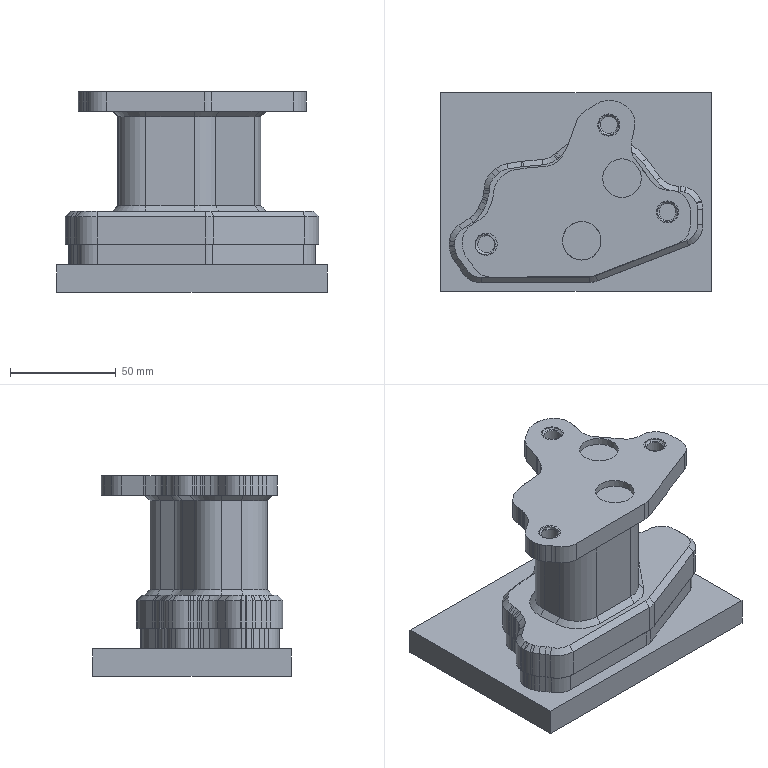NC program | NX | posted by the shop | part box 128.162 x 94.109 x 95 mm
Lines 1 to 893 of 2518:
1 BEGIN PGM B MM
2 BLK FORM 0.1 Z X-200 Y-200 Z-20
3 BLK FORM 0.2  X+200  Y+200  Z+0
4 CYCL DEF 247 DATUM SETTING ~
Q339=+1
5 * - OPERATION: 动态开粗_1_COPY - TOOL: T18 C-D10
6 M5
7 M9
8 PLANE RESET STAY
9 CALL LBL100
10 ;(C-D10 D=10. R=0.)
11 M01
12 TOOL CALL 18 Z S7000
13 CALL LBL101
14 M3 M8
15 M51
16 CYCL DEF 7.0
17 CYCL DEF 7.1 X0
18 CYCL DEF 7.2 Y0
19 CYCL DEF 7.3 Z0
20 CYCL DEF 32.0 TOLERANCE
21 CYCL DEF 32.1 T0.096
22 CYCL DEF 32.2 HSC-MODE:0
23 L M126
24 L A+0.0 C+0.0 FMAX
25 L X65.5231 Y54.6487 FMAX
26 L Z100.1 FMAX
27 L Z85.1 FMAX
28 L Z82.1 F4000.
29 L X65.3697 Y53.0086
30 CC X66.3796 Y52.9169
31 C X65.908 Y52.0191 DR+
32 CC X59.8991 Y27.7131
33 C X68.5518 Y51.2082 DR-
34 CC X64.826 Y44.4706
35 C X72.2902 Y46.3579 DR-
36 CC X43.8286 Y39.0382
37 C X73.2137 Y38.6371 DR-
38 L X73.2796 Y29.0376
39 L X73.2534 Y-44.7659
40 CC X67.0232 Y-43.8302
41 C X69.4184 Y-49.6572 DR-
42 CC X70.3761 Y-52.7478
43 C X67.7081 Y-50.9173 DR+
44 CC X63.6112 Y-46.2833
45 C X65.842 Y-52.0524 DR-
46 CC X66.2949 Y-52.944
47 C X66.2119 Y-53.9406 DR+
48 L X66.8127 Y-53.8771 Z82.2533
49 L X67.4061 Y-53.7642 Z82.4066
50 L X68.1568 Y-53.6324 Z82.6
51 L X69.8793 Y-53.3203 F15000.
52 L X70.1271 Y-53.2006
53 L X72.8269 Y-51.3837
54 CC X68.1598 Y-45.2629
55 C X75.2625 Y-48.229 DR+
56 CC X64.7277 Y-43.3664
57 C X76.3295 Y-43.5273 DR+
58 L X77.2543 Y25.4765
59 CC X-25.2401 Y26.8347
60 C X76.3881 Y40.2005 DR+
61 L X75.6476 Y45.7172
62 CC X62.7408 Y43.3635
63 C X73.232 Y51.2414 DR+
64 CC X65.6303 Y45.2338
65 C X71.4123 Y53.0085 DR+
66 L X69.6105 Y54.3237
67 CC X69.1482 Y53.3821
68 C X68.9718 Y54.4161 DR+
69 L X67.3131 Y54.1061
70 L X66.0198 Y53.8508 Z82.2652 F4000.
71 CC X66.4053 Y52.8551
72 CP IPA34.9502 IZ-.1652 DR+
73 CC X66.3619 Y52.911
74 C X65.908 Y52.0191 DR+
75 CC X62.1689 Y43.8151
76 C X70.2548 Y47.8032 DR-
77 CC X52.9069 Y39.3043
78 C X72.2083 Y40.1037 DR-
79 CC X-136.0307 Y29.0316
80 C X72.4791 Y25.9096 DR-
81 L X72.4538 Y-42.3025
82 CC X64.2353 Y-41.3322
83 C X69.9435 Y-47.3239 DR-
84 CC X71.2981 Y-49.0395
85 C X69.1919 Y-48.4547 DR+
86 CC X62.6392 Y-46.3457
87 C X68.3045 Y-50.256 DR-
88 CC X69.14 Y-50.8056
89 C X69.4411 Y-51.7593 DR+
90 L X69.827 Y-51.5366 Z82.2132
91 L X70.1633 Y-51.2443 Z82.3263
92 L X70.98 Y-50.5415 Z82.6
93 L X72.5067 Y-49.2155 F15000.
94 L X74.4022 Y-46.3635
95 CC X68.1042 Y-42.7162
96 C X75.3794 Y-42.914 DR+
97 L X75.9502 Y-20.9168
98 CC X-709.6475 Y-4.5601
99 C X75.8982 Y14.1254 DR+
100 L X75.1833 Y44.0744
101 CC X67.9863 Y43.899
102 C X73.9781 Y47.8898 DR+
103 L X71.6313 Y51.3912
104 L X71.4675 Y51.528
105 L X71.2861 Y51.6404
106 L X69.7372 Y52.315
107 L X68.2309 Y52.9559 Z82.1844 F4000.
108 L X67.8994 Y52.9814 Z82.1
109 CC X67.9898 Y51.9853
110 C X67.2824 Y51.2783 DR+
111 CC X62.923 Y46.1428
112 C X69.3811 Y48.0589 DR-
113 CC X39.2885 Y36.5453
114 C X71.5034 Y37.12 DR-
115 CC X-338.6129 Y24.7933
116 C X71.6792 Y22.0224 DR-
117 L X71.6451 Y-40.2768
118 CC X58.7607 Y-38.7741
119 C X69.6144 Y-45.8779 DR-
120 CC X71.4265 Y-46.8913
121 C X69.377 Y-47.2235 DR+
122 L X69.1986 Y-48.4101
123 CC X70.1878 Y-48.5585
124 C X70.498 Y-49.5094 DR+
125 CC X70.0128 Y-48.3113
126 CP IPA42.1022 IZ.2409 DR+
127 L X71.7352 Y-48.0227 Z82.6
128 L X72.4667 Y-46.8889 F15000.
129 L X72.5288 Y-46.6825
130 L X72.5603 Y-46.4692
131 L X72.8284 Y47.8111
132 CC X71.8193 Y47.8092
133 C X72.3949 Y48.638 DR+
134 L X71.5444 Y49.2227
135 L X70.4736 Y49.9413 Z82.2724 F4000.
136 CC X70.0492 Y48.9699
137 CP IPA36.7473 IZ-.1724 DR+
138 CC X70.0563 Y49.0323
139 C X69.0789 Y48.8158 DR+
140 CC X-21.6563 Y30.7456
141 C X70.8549 Y29.7066 DR-
142 L X70.8456 Y-38.3927
143 CC X51.6289 Y-36.657
144 C X69.3892 Y-44.198 DR-
145 L X69.3771 Y-46.5972
146 CC X70.3778 Y-46.5964
147 C X70.4616 Y-47.5937 DR+
148 CC X70.3344 Y-46.5054
149 CP IPA55.2046 IZ.2676 DR+
150 L X71.826 Y-46.2733 Z82.6
151 L X72.6354 Y-45.0995 F15000.
152 L X72.7059 Y-44.8823
153 L X72.7388 Y-44.6563
154 L X72.7032 Y45.7946
155 L X72.6372 Y46.011
156 L X72.5363 Y46.2135
157 L X71.8357 Y47.223
158 L X71.0714 Y48.3014 Z82.2643 F4000.
159 CC X70.3195 Y47.5417
160 CP IPA34.7263 IZ-.1643 DR+
161 CC X70.3534 Y47.6053
162 C X69.353 Y47.5845 DR+
163 CC X194.1957 Y48.0079
164 C X69.8207 Y37.2036 DR+
165 CC X-355.6725 Y21.8096
166 C X70.0783 Y17.6074 DR-
167 L X70.0509 Y-36.5922
168 CC X46.6757 Y-35.3927
169 C X69.3772 Y-41.0917 DR-
170 L X69.3771 Y-44.3917
171 CC X70.3771 Y-44.3916
172 C X71.3142 Y-44.7408 DR+
173 L X71.8334 Y-42.8388 Z82.6
174 L X72.0023 Y-42.2488 F15000.
175 L X72.122 Y-41.6468
176 L X72.7411 Y42.1123
177 L X72.6928 Y42.4173
178 L X72.5587 Y42.6955
179 L X71.8363 Y43.7213
180 L X71.0861 Y44.7607 Z82.2744 F4000.
181 CC X70.3531 Y43.9974
182 CP IPA37.2271 IZ-.1744 DR+
183 CC X70.3802 Y44.0524
184 C X69.3794 Y44.0532 DR+
185 L X69.3772 Y-41.1468
186 CC X70.3876 Y-41.1462
187 C X70.6862 Y-42.1115 DR+
188 L X71.1865 Y-41.9481
189 L X71.699 Y-41.828
190 CC X71.7599 Y-42.8361
191 C X71.8408 Y-43.8429 DR-
192 L Z85.1
193 L Z100.1 FMAX
194 L X-63.991 Y-54.784 FMAX
195 L Z85.1 FMAX
196 L Z82.1
197 CC X-64.1911 Y-53.793
198 C X-65.1854 Y-53.9757 DR-
199 L X-65.3121 Y-53.2387
200 L X-65.4789 Y-52.5097
201 CC X-66.4514 Y-52.9474
202 C X-65.9277 Y-52.0184 DR+
203 CC X-57.4511 Y-19.1989
204 C X-68.444 Y-51.2633 DR-
205 CC X-64.7635 Y-44.4368
206 C X-72.2791 Y-46.3506 DR-
207 CC X-43.4503 Y-38.9275
208 C X-73.2153 Y-38.4311 DR-
209 L X-73.2769 Y-29.2315
210 L X-73.2395 Y44.8736
211 CC X-67.0453 Y43.8397
212 C X-69.4858 Y49.626 DR-
213 L X-68.3627 Y50.1762
214 CC X-63.5742 Y46.3859
215 C X-65.9042 Y52.031 DR-
216 CC X-66.3695 Y52.9163
217 C X-66.1448 Y53.8908 DR+
218 L X-66.5885 Y53.8959 Z82.2127
219 L X-67.0252 Y53.8171 Z82.3254
220 L X-68.0904 Y53.6314 Z82.6
221 L X-69.9407 Y53.2992 F15000.
222 L X-70.1894 Y53.1793
223 L X-72.8892 Y51.3624
224 CC X-68.2221 Y45.2416
225 C X-75.3248 Y48.2077 DR+
226 CC X-64.79 Y43.345
227 C X-76.3918 Y43.506 DR+
228 L X-77.267 Y-21.8012
229 CC X59.057 Y-23.611
230 C X-76.408 Y-38.9977 DR+
231 L X-75.6237 Y-45.7678
232 CC X-63.6667 Y-43.8711
233 C X-72.9547 Y-51.6365 DR+
234 CC X-65.6826 Y-45.1881
235 C X-71.4485 Y-53.0123 DR+
236 L X-69.6306 Y-54.3216
237 CC X-69.1731 Y-53.3761
238 C X-68.9954 Y-54.4113 DR+
239 L X-67.3484 Y-54.1012
240 L X-66.0515 Y-53.8436 Z82.2641 F4000.
241 CC X-66.438 Y-52.8469
242 CP IPA34.6972 IZ-.1641 DR+
243 CC X-66.3939 Y-52.9039
244 C X-65.9277 Y-52.0184 DR+
245 CC X-62.0364 Y-43.7205
246 C X-70.2418 Y-47.8031 DR-
247 CC X-52.5413 Y-39.1616
248 C X-72.228 Y-39.8081 DR-
249 CC X191.8602 Y-27.6687
250 C X-72.4772 Y-23.7132 DR-
251 L X-72.4512 Y42.3108
252 CC X-64.3707 Y41.3836
253 C X-70.0232 Y47.2319 DR-
254 CC X-71.5034 Y49.1883
255 C X-69.0786 Y48.8158 DR+
256 CC X-42.6537 Y35.2732
257 C X-68.2967 Y50.2435 DR-
258 CC X-69.0109 Y50.9435
259 C X-69.4178 Y51.857 DR+
260 L X-69.8212 Y51.5726 Z82.2253
261 L X-70.1874 Y51.2416 Z82.3506
262 L X-70.9262 Y50.5935 Z82.6
263 L X-72.5021 Y49.1995 F15000.
264 L X-74.3944 Y46.3512
265 CC X-68.0946 Y42.7028
266 C X-75.3718 Y42.9013 DR+
267 L X-75.943 Y21.413
268 CC X654.4759 Y2.0349
269 C X-75.8641 Y-20.1183 DR+
270 L X-75.105 Y-45.1039
271 CC X-68.9945 Y-44.9149
272 C X-73.897 Y-48.5672 DR+
273 L X-72.9778 Y-49.8177
274 L X-72.0295 Y-51.0462
275 L X-71.7428 Y-51.2359
276 L X-70.1183 Y-51.9453
277 L X-68.7169 Y-52.5452 Z82.2129 F4000.
278 L X-68.4962 Y-52.571 Z82.1564
279 L X-68.2742 Y-52.5627 Z82.1
280 CC X-68.4575 Y-51.5794
281 C X-67.7078 Y-50.9173 DR+
282 CC X-62.6154 Y-46.0911
283 C X-69.3424 Y-48.0843 DR-
284 CC X-39.7381 Y-36.5681
285 C X-71.4981 Y-37.1511 DR-
286 CC X335.7578 Y-24.7604
287 C X-71.6769 Y-21.9536 DR-
288 L X-71.6452 Y40.2458
289 CC X-59.5197 Y38.9909
290 C X-69.7285 Y45.653 DR-
291 CC X-72.3691 Y47.169
292 C X-69.3527 Y47.5845 DR+
293 L X-69.1789 Y48.3654
294 CC X-70.1552 Y48.5825
295 C X-70.5905 Y49.4829 DR+
296 CC X-69.8911 Y48.2692
297 CP IPA34.0662 IZ.2112 DR+
298 L X-71.7638 Y47.9255 Z82.6
299 L X-72.4502 Y46.8357 F15000.
300 L X-72.5094 Y46.6332
301 L X-72.5406 Y46.4245
302 L X-72.9412 Y-47.4501
303 CC X-71.933 Y-47.4499
304 C X-72.4877 Y-48.2917 DR+
305 L X-71.6634 Y-48.8298
306 L X-70.5768 Y-49.5216 Z82.2728 F4000.
307 CC X-70.1763 Y-48.5404
308 CP IPA36.8374 IZ-.1728 DR+
309 CC X-70.1822 Y-48.6023
310 C X-69.1916 Y-48.4547 DR+
311 CC X122.4897 Y-16.6918
312 C X-70.4983 Y-39.192 DR-
313 CC X119.3213 Y-27.0395
314 C X-70.8737 Y-24.8009 DR-
315 L X-70.8433 Y38.3985
316 CC X-50.738 Y36.4406
317 C X-69.3862 Y44.2058 DR-
318 L X-69.3749 Y46.5532
319 CC X-70.3757 Y46.5627
320 C X-70.4256 Y47.5623 DR+
321 CC X-70.3329 Y46.4685
322 CP IPA57.5196 IZ.2794 DR+
323 L X-71.8021 Y46.2658 Z82.6
324 L X-72.634 Y45.0535 F15000.
325 L X-72.7039 Y44.8372
326 L X-72.7366 Y44.6123
327 L X-72.7269 Y-45.4349
328 L X-72.6599 Y-45.6531
329 L X-72.5571 Y-45.8569
330 L X-71.8597 Y-46.8509
331 L X-71.0913 Y-47.9231 Z82.265 F4000.
332 CC X-70.3444 Y-47.1598
333 CP IPA34.9007 IZ-.165 DR+
334 CC X-70.3774 Y-47.2227
335 C X-69.3768 Y-47.2235 DR+
336 CC X-162.5223 Y-46.5544
337 C X-69.7778 Y-37.8945 DR+
338 CC X322.9775 Y-21.9083
339 C X-70.076 Y-17.2995 DR-
340 L X-70.0483 Y36.6002
341 CC X-46.8827 Y35.4081
342 C X-69.3791 Y41.0631 DR-
343 L Y44.3631
344 CC X-70.3792 Y44.3629
345 C X-71.2802 Y44.7968 DR+
346 L X-71.5585 Y43.8514 Z82.35
347 L X-71.8114 Y42.8989 Z82.6
348 L X-72.1148 Y41.7463 F15000.
349 L X-72.7386 Y-42.0826
350 L X-72.6902 Y-42.3875
351 L X-72.5562 Y-42.6657
352 L X-71.8582 Y-43.6568
353 L X-71.0896 Y-44.7249 Z82.2658 F4000.
354 CC X-70.3452 Y-43.9605
355 CP IPA35.1027 IZ-.1658 DR+
356 CC X-70.3775 Y-44.0227
357 C X-69.3769 Y-44.0235 DR+
358 L X-69.3791 Y41.0765
359 CC X-70.3906 Y41.0751
360 C X-70.2437 Y42.076 DR+
361 L X-71.8187 Y42.305
362 L Z85.1
363 L Z100.1 FMAX
364 PLANE RESET STAY
365 * - OPERATION: 动态开粗_1 - TOOL: T18 C-D10
366 CYCL DEF 32.0 TOLERANCE
367 CYCL DEF 32.1 T0.096
368 CYCL DEF 32.2 HSC-MODE:0
369 L A+0.0 C+0.0 FMAX
370 L X71.6405 Y1.4365 FMAX
371 L Z100. FMAX
372 L Z75.5361 FMAX
373 L Z72.5361 F4000.
374 L X69.6182 Y.4541
375 CC X70.1084 Y-.5042
376 C X69.1596 Y.0041 DR+
377 CC X79.1767 Y-3.8411
378 C X68.447 Y-3.8787 DR+
379 CC X361.5552 Y-13.7916
380 C X68.2801 Y-14.4035 DR+
381 L X68.2535 Y-44.7659
382 CC X62.0101 Y-43.8266
383 C X64.4238 Y-49.6607 DR-
384 CC X57.2669 Y-32.5753
385 C X57.4167 Y-51.0985 DR-
386 CC X47.0047 Y296.47
387 C X45.619 Y-51.2516 DR-
388 L X-61.9391 Y-51.212
389 CC X-60.7765 Y-44.9278
390 C X-66.6716 Y-47.3956 DR-
391 CC X-49.8833 Y-40.2742
392 C X-68.1183 Y-40.4897 DR-
393 CC X282.7887 Y-29.4374
394 C X-68.28 Y-26.4921 DR-
395 L X-68.2418 Y44.8737
396 CC X-61.9527 Y43.7878
397 C X-64.3299 Y49.7107 DR-
398 CC X-57.2383 Y32.335
399 C X-57.4121 Y51.1014 DR-
400 CC X-46.9584 Y-302.6918
401 C X-45.6143 Y51.2532 DR-
402 L X61.8004 Y51.227
403 CC X60.8663 Y45.0048
404 C X66.6494 Y47.4835 DR-
405 CC X49.8278 Y40.2787
406 C X68.1271 Y40.3857 DR-
407 CC X-282.7002 Y29.9586
408 C X68.2793 Y28.5879 DR-
409 L X68.249 Y2.3886
410 CC X198.4264 Y-11.8206
411 C X67.4868 Y-13.5142 DR+
412 L X67.4539 Y-42.3026
413 CC X59.6658 Y-41.4074
414 C X62.6904 Y-48.6398 DR-
415 CC X54.5689 Y-29.2309
416 C X54.9086 Y-50.2677 DR-
417 CC X44.3375 Y244.9354
418 C X42.5115 Y-50.4513 DR-
419 L X-59.3761 Y-50.4204
420 CC X-58.3699 Y-42.5497
421 C X-65.7345 Y-45.503 DR-
422 CC X-45.4319 Y-37.3485
423 C X-67.3095 Y-37.6029 DR-
424 CC X261.3603 Y-26.9474
425 C X-67.479 Y-25.5054 DR-
426 L X-67.4533 Y42.3108
427 CC X-59.6835 Y41.4196
428 C X-62.7468 Y48.6155 DR-
429 CC X-54.7168 Y29.807
430 C X-55.1704 Y50.2529 DR-
431 CC X-43.5644 Y-256.7811
432 C X-40.1739 Y50.4535 DR-
433 L X59.3369 Y50.4268
434 CC X58.4393 Y42.6413
435 C X65.6704 Y45.6631 DR-
436 CC X46.2537 Y37.5472
437 C X67.2957 Y37.8801 DR-
438 CC X-247.5041 Y26.8258
439 C X67.4794 Y24.283 DR-
440 CC X-847.4335 Y16.3748
441 C X67.4202 Y3.2976 DR-
442 CC X300.432 Y-15.6072
443 C X66.6792 Y-19.0031 DR+
444 CC X-911.3933 Y-27.7345
445 C X66.6361 Y-40.402 DR-
446 CC X57.7611 Y-39.502
447 C X61.067 Y-47.7874 DR-
448 CC X52.2992 Y-25.7183
449 C X52.6809 Y-49.4622 DR-
450 CC X41.5999 Y263.7296
451 C X39.4838 Y-49.651 DR-
452 L X-57.2156 Y-49.6228
453 CC X-56.5163 Y-40.7134
454 C X-64.8381 Y-43.9714 DR-
455 CC X-42.3082 Y-35.158
456 C X-66.4985 Y-35.4797 DR-
457 CC X285.409 Y-23.9192
458 C X-66.6792 Y-21.3824 DR-
459 L X-66.643 Y40.3167
460 CC X-57.7969 Y39.5269
461 C X-61.1651 Y47.7448 DR-
462 CC X-52.3747 Y26.0973
463 C X-52.783 Y49.4579 DR-
464 CC X-40.6821 Y-295.902
465 C X-37.2861 Y49.6531 DR-
466 L X57.3131 Y49.619
467 CC X56.5339 Y40.7317
468 C X64.8382 Y43.9921 DR-
469 CC X42.3393 Y35.1845
470 C X66.4986 Y35.5013 DR-
471 CC X-287.0018 Y23.9034
472 C X66.6792 Y21.304 DR-
473 CC X-469.0986 Y15.3826
474 C X66.5779 Y3.3985 DR-
475 CC X345.3128 Y-16.5419
476 C X65.8802 Y-19.4051 DR+
477 CC X-793.8738 Y-26.5384
478 C X65.8238 Y-38.7028 DR-
479 CC X56.1711 Y-37.8919
480 C X59.7658 Y-46.8869 DR-
481 CC X50.5117 Y-23.4883
482 C X50.9853 Y-48.646 DR-
483 CC X38.7119 Y291.3707
484 C X35.3886 Y-48.8512 DR-
485 L X-55.4108 Y-48.8167
486 CC X-54.9003 Y-39.1249
487 C X-63.9103 Y-42.7324 DR-
488 CC X-40.5069 Y-33.469
489 C X-65.6722 Y-33.9543 DR-
490 CC X269.3953 Y-21.7378
491 C X-65.8788 Y-18.4576 DR-
492 L X-65.8425 Y38.4417
493 CC X-56.1393 Y37.878
494 C X-59.6337 Y46.9477 DR-
495 CC X-50.527 Y23.3661
496 C X-51.1379 Y48.6377 DR-
497 CC X-38.8269 Y-276.9229
498 C X-35.4415 Y48.8527 DR-
499 L X55.358 Y48.8227
500 CC X54.9163 Y39.142
501 C X63.9203 Y42.7252 DR-
502 CC X40.2638 Y33.4225
503 C X65.6801 Y33.848 DR-
504 CC X-244.6344 Y22.5882
505 C X65.8783 Y20.6511 DR-
506 CC X-310.8721 Y15.2421
507 C X65.7034 Y2.5543 DR-
508 CC X376.7183 Y-17.2407
509 C X65.0803 Y-19.2049 DR+
510 CC X-541.9694 Y-25.8315
511 C X65.01 Y-37.2021 DR-
512 CC X54.6518 Y-36.3917
513 C X58.2574 Y-46.1358 DR-
514 CC X48.6537 Y-20.1548
515 C X49.1623 Y-47.8493 DR-
516 CC X36.6826 Y312.8662
517 C X33.4654 Y-48.0508 DR-
518 L X-53.7764 Y-48.0118
519 CC X-53.4082 Y-37.6336
520 C X-63.1024 Y-41.3574 DR-
521 CC X-37.8116 Y-31.7301
522 C X-64.8673 Y-32.2743 DR-
523 CC X285.8471 Y-19.6023
524 C X-65.0785 Y-16.0776 DR-
525 L X-65.0522 Y36.522
526 CC X-54.6596 Y36.3818
527 C X-58.3547 Y46.0964 DR-
528 CC X-48.9233 Y21.3095
529 C X-49.6669 Y47.8196 DR-
530 CC X-37.0838 Y-265.7701
531 C X-33.5709 Y48.0523 DR-
532 L X53.7285 Y48.0172
533 CC X53.3948 Y37.5984
534 C X63.1948 Y41.1511 DR-
535 CC X37.1927 Y31.648
536 C X64.8705 Y32.2429 DR-
537 CC X-406.1117 Y17.0858
538 C X64.9023 Y2.949 DR-
539 CC X434.7168 Y-18.6577
540 C X64.2797 Y-21.104 DR+
541 CC X-327.6751 Y-26.278
542 C X64.1981 Y-35.802 DR-
543 CC X53.2956 Y-35.0272
544 C X57.0494 Y-45.2924 DR-
545 CC X47.2454 Y-18.5641
546 C X47.9538 Y-47.025 DR-
547 CC X34.9944 Y294.2995
548 C X31.2575 Y-47.2505 DR-
549 L X-52.142 Y-47.2134
550 CC X-52.0155 Y-36.245
551 C X-62.3027 Y-40.0524 DR-
552 CC X-35.9286 Y-30.2827
553 C X-64.0433 Y-31.0612 DR-
554 CC X262.9895 Y-18.088
555 C X-64.2781 Y-14.2652 DR-
556 L X-64.2459 Y35.0344
557 CC X-53.2276 Y34.9686
558 C X-56.8531 Y45.3737 DR-
559 CC X-47.063 Y17.5699
560 C X-47.7406 Y47.0391 DR-
561 CC X-34.8243 Y-314.5893
562 C X-31.2439 Y47.252 DR-
563 L X52.0557 Y47.2198
564 CC X52.0018 Y36.2185
565 C X62.3639 Y39.9143 DR-
566 CC X34.6968 Y30.0291
567 C X64.071 Y30.6122 DR-
568 CC X-356.0922 Y16.689
569 C X63.676 Y-6.2379 DR-
570 CC X1030.0374 Y-27.5321
571 C X63.4581 Y-33.2027 DR+
572 CC X51.7056 Y-33.5522
573 C X60.2182 Y-41.6626 DR-
574 CC X49.7455 Y-30.2677
575 C X52.1134 Y-45.5619 DR-
576 CC X41.442 Y20.6017
577 C X40.5599 Y-46.4112 DR-
578 L X-50.5395 Y-46.417
579 CC X-50.6823 Y-34.9175
580 C X-61.5127 Y-38.7855 DR-
581 CC X-32.9212 Y-28.6173
582 C X-63.2596 Y-29.2833 DR-
583 CC X291.5364 Y-16.4281
584 C X-63.4777 Y-13.1867 DR-
585 L X-63.4414 Y33.6128
586 CC X-51.9458 Y33.6678
587 C X-55.7452 Y44.5175 DR-
588 CC X-45.543 Y15.3381
589 C X-46.1387 Y46.2439 DR-
590 CC X-33.3256 Y-326.0479
591 C X-30.2418 Y46.4515 DR-
592 L X50.4579 Y46.4227
593 CC X50.6885 Y34.9388
594 C X61.4621 Y38.9215 DR-
595 CC X33.9225 Y28.8366
596 C X63.2398 Y29.6298 DR-
597 CC X-313.6544 Y15.6733
598 C X62.9174 Y-5.2478 DR-
599 CC X935.9996 Y-27.1249
600 C X62.6559 Y-31.804 DR+
601 CC X49.9196 Y-32.1673
602 C X60.0929 Y-39.8387 DR-
603 CC X49.27 Y-30.3996
604 C X52.182 Y-44.462 DR-
605 CC X41.6325 Y5.394
606 C X41.4591 Y-45.5656 DR-
607 L X30.0597 Y-45.6491
608 L X-49.04 Y-45.619
609 CC X-49.2963 Y-33.2532
610 C X-57.3458 Y-42.6439 DR-
611 CC X-46.8069 Y-31.8913
612 C X-61.6132 Y-34.6223 DR-
613 CC X-4.3421 Y-23.8321
614 C X-62.6183 Y-23.2859 DR-
615 L X-62.6768 Y-12.9863
616 L X-62.6396 Y32.2133
617 CC X-50.6598 Y32.3998
618 C X-58.8849 Y41.1118 DR-
619 CC X-48.1931 Y28.2889
620 C X-50.4794 Y44.8272 DR-
621 CC X-39.1036 Y-34.4531
622 C X-37.7184 Y45.6272 DR-
623 L X49.281 Y45.6115
624 CC X49.4431 Y33.6815
625 C X58.3389 Y41.6323 DR-
626 CC X44.9508 Y31.0166
627 C X61.8901 Y33.251 DR-
628 CC X-21.2412 Y21.848
629 C X62.6559 Y20.3874 DR-
630 CC X-377.633 Y16.4874
631 C X62.0968 Y-6.0333 DR-
632 CC X981.3229 Y-27.6815
633 C X61.8469 Y-30.704 DR+
634 CC X48.6497 Y-30.9713
635 C X59.308 Y-38.7584 DR-
636 CC X48.1221 Y-29.2703
637 C X51.0547 Y-43.6421 DR-
638 CC X40.1832 Y8.2559
639 C X39.9333 Y-44.7679 DR-
640 L X26.6339 Y-44.8493
641 L X-47.6658 Y-44.8184
642 CC X-47.9644 Y-31.5243
643 C X-55.672 Y-42.3602 DR-
644 CC X-46.5225 Y-31.2376
645 C X-60.5862 Y-34.3417 DR-
646 CC X-12.1363 Y-23.4971
647 C X-61.7848 Y-23.3298 DR-
648 L X-61.8764 Y-11.6305
649 L X-61.8491 Y30.5693
650 CC X-48.4572 Y30.9147
651 C X-59.4481 Y38.5739 DR-
652 CC X-48.315 Y29.5728
653 C X-51.4199 Y43.5486 DR-
654 CC X-40.6281 Y-4.1281
655 C X-40.51 Y44.7546 DR-
656 CC X-29.0089 Y-609.9626
657 C X-26.5107 Y44.8508 DR-
658 L X47.6889 Y44.8197
659 CC X47.9911 Y31.6199
660 C X55.8412 Y42.236 DR-
661 CC X46.3647 Y31.1485
662 C X60.6318 Y34.1794 DR-
663 CC X9.5629 Y23.2039
664 C X61.7968 Y22.8628 DR-
665 CC X-389.3944 Y16.017
666 C X61.2903 Y-6.4262 DR-
667 CC X939.4913 Y-27.2504
668 C X61.046 Y-29.4042 DR+
669 CC X47.028 Y-29.6976
670 C X58.7174 Y-37.4402 DR-
671 CC X47.2692 Y-28.5722
672 C X50.425 Y-42.7053 DR-
673 CC X39.4073 Y5.501
674 C X39.3184 Y-43.9482 DR-
675 CC X28.0931 Y580.0297
676 C X27.0191 Y-44.0483 DR-
677 L X-46.3806 Y-44.0168
678 CC X-46.6798 Y-29.8021
679 C X-54.1827 Y-41.879 DR-
680 CC X-45.9093 Y-30.4482
681 C X-59.6046 Y-33.8473 DR-
682 CC X-16.4387 Y-23.0031
683 C X-60.9451 Y-23.2586 DR-
684 CC X558.8359 Y-10.5257
685 C X-61.0759 Y-10.3598 DR-
686 L X-61.0387 Y29.5398
687 CC X-47.3587 Y29.7895
688 C X-58.5096 Y37.718 DR-
689 CC X-47.0938 Y28.2933
690 C X-50.1577 Y42.7763 DR-
691 CC X-38.9683 Y-9.149
692 C X-38.6432 Y43.9673 DR-
693 L X-27.4438 Y44.0497
694 L X46.5558 Y44.0127
695 CC X46.8055 Y30.2911
696 C X54.7334 Y41.4934 DR-
697 CC X45.4529 Y30.1674
698 C X59.7439 Y33.3572 DR-
699 CC X9.823 Y22.1391
700 C X60.988 Y21.8502 DR-
701 CC X-362.3882 Y15.2924
702 C X60.5166 Y-5.7305 DR-
703 CC X1010.6387 Y-28.8292
704 C X60.2359 Y-28.4048 DR+
705 CC X46.0104 Y-28.6173
706 C X57.782 Y-36.6072 DR-
707 CC X46.2282 Y-27.5175
708 C X49.5626 Y-41.8351 DR-
709 CC X38.6049 Y4.1505
710 C X38.8642 Y-43.1219 DR-
711 CC X26.3533 Y577.9921
712 C X25.9654 Y-43.2478 DR-
713 L X-45.0344 Y-43.2181
714 CC X-45.4098 Y-28.0985
715 C X-52.9737 Y-41.1955 DR-
716 CC X-45.0481 Y-29.5211
717 C X-58.7079 Y-33.059 DR-
718 CC X-16.7459 Y-22.037
719 C X-60.1299 Y-22.3801 DR-
720 CC X562.1926 Y-8.9225
721 C X-60.2754 Y-8.9816 DR-
722 L X-60.2433 Y28.1181
723 CC X-45.3569 Y28.4514
724 C X-58.167 Y36.042 DR-
725 CC X-46.4783 Y27.9263
726 C X-49.9423 Y41.7282 DR-
727 CC X-38.6482 Y-3.0512
728 C X-38.6591 Y43.1305 DR-
729 CC X-25.9933 Y-610.6425
730 C X-23.9602 Y43.25 DR-
731 L X45.0396 Y43.2201
732 CC X45.4091 Y27.9912
733 C X52.8095 Y41.3062 DR-
734 CC X45.1432 Y29.5865
735 C X58.6961 Y33.1138 DR-
736 CC X17.8004 Y22.2317
737 C X60.1161 Y22.7385 DR-
738 CC X-291.0453 Y13.7673
739 C X59.7688 Y-4.2413 DR-
740 CC X957.3036 Y-28.7607
741 C X59.4353 Y-27.2078 DR+
742 CC X44.444 Y-27.4194
743 C X57.2046 Y-35.2902 DR-
744 CC X45.373 Y-26.7654
745 C X48.9041 Y-40.9142 DR-
746 CC X37.5735 Y4.0915
747 C X37.7207 Y-42.3184 DR-
748 CC X24.2031 Y635.7105
749 C X21.6219 Y-42.4482 DR-
750 L X-43.8778 Y-42.4152
751 CC X-44.2424 Y-26.6229
752 C X-51.8472 Y-40.4684 DR-
753 CC X-44.1182 Y-28.5607
754 C X-57.8321 Y-32.2295 DR-
755 CC X-16.4776 Y-21.0402
756 C X-59.317 Y-21.4619 DR-
757 CC X527.3466 Y-7.8425
758 C X-59.475 Y-7.6636 DR-
759 L X-59.4344 Y27.136
760 CC X-44.2877 Y27.3835
761 C X-57.2967 Y35.1456 DR-
762 CC X-45.5133 Y26.9599
763 C X-49.1997 Y40.8259 DR-
764 CC X-37.9709 Y-1.2287
765 C X-38.3291 Y42.2977 DR-
766 CC X-24.5751 Y-582.4363
767 C X-24.5307 Y42.449 DR-
768 L X43.769 Y42.4202
769 CC X44.1725 Y26.2313
770 C X51.5827 Y40.6304 DR-
771 CC X44.343 Y28.74
772 C X57.7228 Y32.5838 DR-
773 CC X17.9102 Y21.2088
774 C X59.3147 Y21.5331 DR-
775 CC X-280.5512 Y13.1763
776 C X58.9711 Y-4.2375 DR-
777 CC X910.9274 Y-28.2235
778 C X58.6364 Y-26.0108 DR+
779 CC X42.9385 Y-26.2443
780 C X56.5132 Y-34.1314 DR-
781 CC X44.4955 Y-25.952
782 C X48.1833 Y-40.0135 DR-
783 CC X36.6246 Y3.9296
784 C X36.8118 Y-41.5079 DR-
785 CC X22.8866 Y632.7439
786 C X20.6132 Y-41.6478 DR-
787 L X-42.6865 Y-41.6146
788 CC X-43.0573 Y-24.9608
789 C X-50.5991 Y-39.8136 DR-
790 CC X-43.289 Y-27.6794
791 C X-56.9318 Y-31.4941 DR-
792 CC X-16.7169 Y-20.1403
793 C X-58.5008 Y-20.6397 DR-
794 CC X449.9282 Y-7.3001
795 C X-58.6747 Y-6.2417 DR-
796 L X-58.6365 Y25.8579
797 CC X-42.5525 Y26.1623
798 C X-56.6455 Y33.9196 DR-
799 CC X-44.5288 Y26.0158
800 C X-48.1981 Y40.0094 DR-
801 CC X-36.781 Y-3.0074
802 C X-37.1263 Y41.4974 DR-
803 CC X-23.2012 Y-593.1379
804 C X-22.0279 Y41.6491 DR-
805 L X42.5719 Y41.6194
806 CC X43.013 Y24.7329
807 C X50.5061 Y39.8724 DR-
808 CC X43.3669 Y27.7484
809 C X56.8884 Y31.6378 DR-
810 CC X18.0373 Y20.3667
811 C X58.4855 Y20.9879 DR-
812 CC X-245.625 Y12.3779
813 C X58.2061 Y-3.2416 DR-
814 CC X965.0283 Y-29.8996
815 C X57.827 Y-25.1183 DR+
816 CC X42.0711 Y-25.2581
817 C X55.6056 Y-33.3256 DR-
818 CC X43.4779 Y-24.9136
819 C X47.2472 Y-39.1837 DR-
820 CC X35.8911 Y3.1998
821 C X36.4788 Y-40.6747 DR-
822 CC X22.0306 Y536.3187
823 C X18.9808 Y-40.8476 DR-
824 L X-41.7188 Y-40.8079
825 CC X-42.0249 Y-23.8915
826 C X-49.6333 Y-39.0034 DR-
827 CC X-42.3239 Y-26.7111
828 C X-56.0775 Y-30.6313 DR-
829 CC X-16.2269 Y-19.1738
830 C X-57.6873 Y-19.7834 DR-
831 CC X409.4837 Y-6.4579
832 C X-57.8744 Y-4.7857 DR-
833 L X-57.8355 Y24.714
834 CC X-41.1355 Y25.0383
835 C X-55.9255 Y32.8004 DR-
836 CC X-43.6725 Y25.2027
837 C X-47.5435 Y39.0907 DR-
838 CC X-36.2043 Y-.9877
839 C X-36.888 Y40.6582 DR-
840 CC X-23.2628 Y-429.1236
841 C X-20.6904 Y40.8487 DR-
842 L X41.5094 Y40.8161
843 CC X41.9142 Y23.3859
844 C X49.4499 Y39.1081 DR-
845 CC X42.4126 Y26.7759
846 C X56.0589 Y30.6987 DR-
847 CC X16.7203 Y19.2647
848 C X57.6827 Y19.8536 DR-
849 CC X-248.3054 Y11.8884
850 C X57.3974 Y-3.536 DR-
851 CC X989.4659 Y-30.7622
852 C X57.0235 Y-24.1255 DR+
853 CC X40.9789 Y-24.2229
854 C X54.7738 Y-32.4168 DR-
855 CC X42.4333 Y-23.8559
856 C X46.1439 Y-38.4095 DR-
857 CC X34.3415 Y7.4226
858 C X34.5709 Y-39.9042 DR-
859 CC X20.3026 Y647.4461
860 C X17.6723 Y-40.0473 DR-
861 L X-40.6273 Y-40.0059
862 CC X-40.9514 Y-22.6527
863 C X-48.7366 Y-38.1649 DR-
864 CC X-41.3218 Y-25.7178
865 C X-55.2555 Y-29.688 DR-
866 CC X-14.7266 Y-18.0562
867 C X-56.8876 Y-18.6419 DR-
868 CC X441.7738 Y-4.7416
869 C X-57.0745 Y-2.1442 DR-
870 L X-57.0355 Y23.5555
871 CC X-39.5886 Y23.9054
872 C X-55.2161 Y31.6706 DR-
873 CC X-42.8036 Y24.3614
874 C X-46.8618 Y38.1825 DR-
875 CC X-35.1131 Y-1.9371
876 C X-35.6168 Y39.8644 DR-
877 CC X-21.2463 Y-492.065
878 C X-18.019 Y40.0487 DR-
879 L X40.5806 Y40.0092
880 CC X40.9323 Y22.5623
881 C X48.6966 Y38.1903 DR-
882 CC X41.3798 Y25.7638
883 C X55.2403 Y29.7436 DR-
884 CC X14.8538 Y18.0812
885 C X56.8884 Y18.4978 DR-
886 CC X-257.6755 Y11.5252
887 C X56.5858 Y-3.9306 DR-
888 CC X983.1962 Y-30.8884
889 C X56.2271 Y-23.0331 DR+
890 CC X39.6138 Y-23.1284
891 C X54.0488 Y-31.3528 DR-
892 CC X41.5887 Y-23.0452